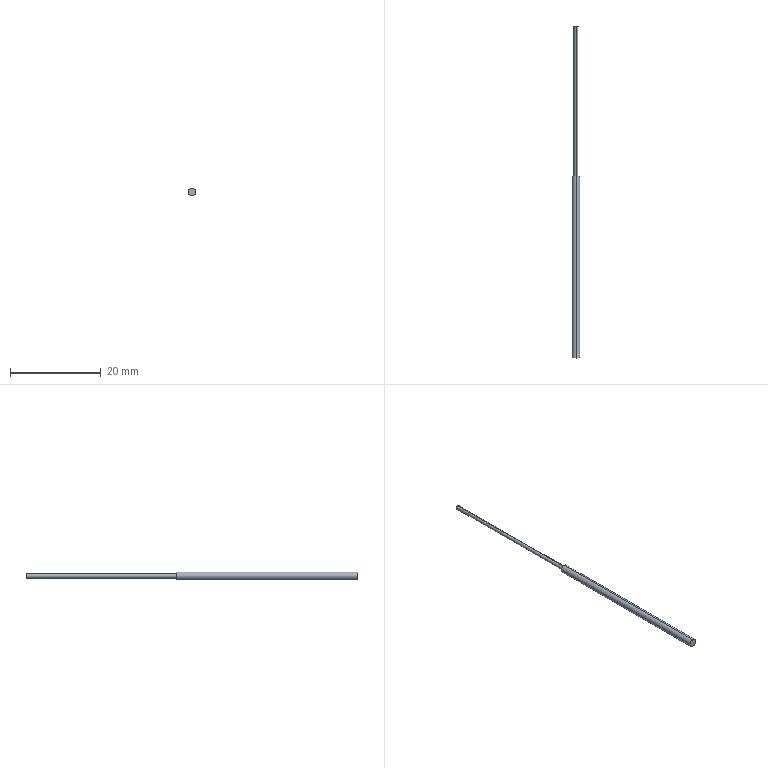Part | SolidWorks | features Extrusion 1, ICE 1 | 1 solid | 7 faces | box 1.75 x 73 x 1.75 mm | volume 117.205 mm3 | cylinder 4 | plane 3 | commonest cylinder face diameters 0.9 x2 1.75 x2
STEP:
#1=CARTESIAN_POINT('',(0.,73.,0.45));
#2=VERTEX_POINT('',#1);
#3=CARTESIAN_POINT('',(0.,73.,-0.45));
#4=VERTEX_POINT('',#3);
#5=CARTESIAN_POINT('',(0.,73.,0.));
#6=DIRECTION('',(0.,1.,0.));
#7=DIRECTION('',(0.,0.,1.));
#8=AXIS2_PLACEMENT_3D('',#5,#6,#7);
#9=CIRCLE('',#8,0.45);
#10=EDGE_CURVE('',#2,#4,#9,.T.);
#11=ORIENTED_EDGE('',*,*,#10,.F.);
#12=CARTESIAN_POINT('',(0.,40.,0.45));
#13=VERTEX_POINT('',#12);
#14=CARTESIAN_POINT('',(0.,73.,0.45));
#15=DIRECTION('',(0.,-1.,0.));
#16=VECTOR('',#15,1000.);
#17=LINE('',#14,#16);
#18=EDGE_CURVE('',#2,#13,#17,.T.);
#19=ORIENTED_EDGE('',*,*,#18,.T.);
#20=CARTESIAN_POINT('',(0.,40.,-0.45));
#21=VERTEX_POINT('',#20);
#22=CARTESIAN_POINT('',(0.,40.,0.));
#23=DIRECTION('',(0.,1.,0.));
#24=DIRECTION('',(0.,0.,1.));
#25=AXIS2_PLACEMENT_3D('',#22,#23,#24);
#26=CIRCLE('',#25,0.45);
#27=EDGE_CURVE('',#13,#21,#26,.T.);
#28=ORIENTED_EDGE('',*,*,#27,.T.);
#29=CARTESIAN_POINT('',(0.,73.,-0.45));
#30=DIRECTION('',(0.,-1.,0.));
#31=VECTOR('',#30,1000.);
#32=LINE('',#29,#31);
#33=EDGE_CURVE('',#4,#21,#32,.T.);
#34=ORIENTED_EDGE('',*,*,#33,.F.);
#35=EDGE_LOOP('',(#11,#19,#28,#34));
#36=FACE_OUTER_BOUND('',#35,.T.);
#37=CARTESIAN_POINT('',(0.,73.,0.));
#38=DIRECTION('',(0.,-1.,0.));
#39=DIRECTION('',(0.,0.,-1.));
#40=AXIS2_PLACEMENT_3D('',#37,#38,#39);
#41=CYLINDRICAL_SURFACE('',#40,0.45);
#42=ADVANCED_FACE('',(#36),#41,.T.);
#43=CARTESIAN_POINT('',(0.,40.,0.875));
#44=VERTEX_POINT('',#43);
#45=CARTESIAN_POINT('',(0.,40.,-0.875));
#46=VERTEX_POINT('',#45);
#47=CARTESIAN_POINT('',(0.,40.,0.));
#48=DIRECTION('',(0.,1.,0.));
#49=DIRECTION('',(0.,0.,1.));
#50=AXIS2_PLACEMENT_3D('',#47,#48,#49);
#51=CIRCLE('',#50,0.875);
#52=EDGE_CURVE('',#44,#46,#51,.T.);
#53=ORIENTED_EDGE('',*,*,#52,.F.);
#54=CARTESIAN_POINT('',(0.,0.,0.875));
#55=VERTEX_POINT('',#54);
#56=CARTESIAN_POINT('',(0.,40.,0.875));
#57=DIRECTION('',(0.,-1.,0.));
#58=VECTOR('',#57,1000.);
#59=LINE('',#56,#58);
#60=EDGE_CURVE('',#44,#55,#59,.T.);
#61=ORIENTED_EDGE('',*,*,#60,.T.);
#62=CARTESIAN_POINT('',(0.,0.,-0.875));
#63=VERTEX_POINT('',#62);
#64=CARTESIAN_POINT('',(0.,0.,0.));
#65=DIRECTION('',(0.,1.,0.));
#66=DIRECTION('',(0.,0.,1.));
#67=AXIS2_PLACEMENT_3D('',#64,#65,#66);
#68=CIRCLE('',#67,0.875);
#69=EDGE_CURVE('',#55,#63,#68,.T.);
#70=ORIENTED_EDGE('',*,*,#69,.T.);
#71=CARTESIAN_POINT('',(0.,40.,-0.875));
#72=DIRECTION('',(0.,-1.,0.));
#73=VECTOR('',#72,1000.);
#74=LINE('',#71,#73);
#75=EDGE_CURVE('',#46,#63,#74,.T.);
#76=ORIENTED_EDGE('',*,*,#75,.F.);
#77=EDGE_LOOP('',(#53,#61,#70,#76));
#78=FACE_OUTER_BOUND('',#77,.T.);
#79=CARTESIAN_POINT('',(0.,40.,0.));
#80=DIRECTION('',(0.,-1.,0.));
#81=DIRECTION('',(0.,0.,-1.));
#82=AXIS2_PLACEMENT_3D('',#79,#80,#81);
#83=CYLINDRICAL_SURFACE('',#82,0.875);
#84=ADVANCED_FACE('',(#78),#83,.T.);
#85=CARTESIAN_POINT('',(0.,40.,0.));
#86=DIRECTION('',(0.,1.,0.));
#87=DIRECTION('',(0.,0.,1.));
#88=AXIS2_PLACEMENT_3D('',#85,#86,#87);
#89=CIRCLE('',#88,0.875);
#90=EDGE_CURVE('',#46,#44,#89,.T.);
#91=ORIENTED_EDGE('',*,*,#90,.T.);
#92=ORIENTED_EDGE('',*,*,#52,.T.);
#93=EDGE_LOOP('',(#91,#92));
#94=FACE_OUTER_BOUND('',#93,.T.);
#95=CARTESIAN_POINT('',(0.,40.,0.));
#96=DIRECTION('',(0.,1.,0.));
#97=DIRECTION('',(0.,0.,1.));
#98=AXIS2_PLACEMENT_3D('',#95,#96,#97);
#99=CIRCLE('',#98,0.45);
#100=EDGE_CURVE('',#21,#13,#99,.T.);
#101=ORIENTED_EDGE('',*,*,#100,.F.);
#102=ORIENTED_EDGE('',*,*,#27,.F.);
#103=EDGE_LOOP('',(#101,#102));
#104=FACE_BOUND('',#103,.T.);
#105=CARTESIAN_POINT('',(0.,40.,0.));
#106=DIRECTION('',(0.,1.,0.));
#107=DIRECTION('',(0.,0.,1.));
#108=AXIS2_PLACEMENT_3D('',#105,#106,#107);
#109=PLANE('',#108);
#110=ADVANCED_FACE('',(#94,#104),#109,.T.);
#111=ORIENTED_EDGE('',*,*,#60,.F.);
#112=ORIENTED_EDGE('',*,*,#90,.F.);
#113=ORIENTED_EDGE('',*,*,#75,.T.);
#114=CARTESIAN_POINT('',(0.,0.,0.));
#115=DIRECTION('',(0.,1.,0.));
#116=DIRECTION('',(0.,0.,1.));
#117=AXIS2_PLACEMENT_3D('',#114,#115,#116);
#118=CIRCLE('',#117,0.875);
#119=EDGE_CURVE('',#63,#55,#118,.T.);
#120=ORIENTED_EDGE('',*,*,#119,.T.);
#121=EDGE_LOOP('',(#111,#112,#113,#120));
#122=FACE_OUTER_BOUND('',#121,.T.);
#123=CARTESIAN_POINT('',(0.,40.,0.));
#124=DIRECTION('',(0.,-1.,0.));
#125=DIRECTION('',(0.,0.,-1.));
#126=AXIS2_PLACEMENT_3D('',#123,#124,#125);
#127=CYLINDRICAL_SURFACE('',#126,0.875);
#128=ADVANCED_FACE('',(#122),#127,.T.);
#129=ORIENTED_EDGE('',*,*,#119,.F.);
#130=ORIENTED_EDGE('',*,*,#69,.F.);
#131=EDGE_LOOP('',(#129,#130));
#132=FACE_OUTER_BOUND('',#131,.T.);
#133=CARTESIAN_POINT('',(0.,0.,0.));
#134=DIRECTION('',(0.,1.,0.));
#135=DIRECTION('',(0.,0.,1.));
#136=AXIS2_PLACEMENT_3D('',#133,#134,#135);
#137=PLANE('',#136);
#138=ADVANCED_FACE('',(#132),#137,.F.);
#139=ORIENTED_EDGE('',*,*,#18,.F.);
#140=CARTESIAN_POINT('',(0.,73.,0.));
#141=DIRECTION('',(0.,1.,0.));
#142=DIRECTION('',(0.,0.,1.));
#143=AXIS2_PLACEMENT_3D('',#140,#141,#142);
#144=CIRCLE('',#143,0.45);
#145=EDGE_CURVE('',#4,#2,#144,.T.);
#146=ORIENTED_EDGE('',*,*,#145,.F.);
#147=ORIENTED_EDGE('',*,*,#33,.T.);
#148=ORIENTED_EDGE('',*,*,#100,.T.);
#149=EDGE_LOOP('',(#139,#146,#147,#148));
#150=FACE_OUTER_BOUND('',#149,.T.);
#151=CARTESIAN_POINT('',(0.,73.,0.));
#152=DIRECTION('',(0.,-1.,0.));
#153=DIRECTION('',(0.,0.,-1.));
#154=AXIS2_PLACEMENT_3D('',#151,#152,#153);
#155=CYLINDRICAL_SURFACE('',#154,0.45);
#156=ADVANCED_FACE('',(#150),#155,.T.);
#157=ORIENTED_EDGE('',*,*,#145,.T.);
#158=ORIENTED_EDGE('',*,*,#10,.T.);
#159=EDGE_LOOP('',(#157,#158));
#160=FACE_OUTER_BOUND('',#159,.T.);
#161=CARTESIAN_POINT('',(0.,73.,0.));
#162=DIRECTION('',(0.,1.,0.));
#163=DIRECTION('',(0.,0.,1.));
#164=AXIS2_PLACEMENT_3D('',#161,#162,#163);
#165=PLANE('',#164);
#166=ADVANCED_FACE('',(#160),#165,.T.);
#167=CLOSED_SHELL('',(#42,#84,#110,#128,#138,#156,#166));
#168=MANIFOLD_SOLID_BREP('',#167);
#169=CARTESIAN_POINT('',(0.,0.,0.));
#170=DIRECTION('',(0.,0.,1.));
#171=DIRECTION('',(1.,0.,0.));
#172=AXIS2_PLACEMENT_3D('',#169,#170,#171);
#173=(LENGTH_UNIT()NAMED_UNIT(*)SI_UNIT(.MILLI.,.METRE.));
#174=UNCERTAINTY_MEASURE_WITH_UNIT(LENGTH_MEASURE(0.00001),#173,'','');
#175=(NAMED_UNIT(*)PLANE_ANGLE_UNIT()SI_UNIT($,.RADIAN.));
#176=(NAMED_UNIT(*)SI_UNIT($,.STERADIAN.)SOLID_ANGLE_UNIT());
#177=(GEOMETRIC_REPRESENTATION_CONTEXT(3)GLOBAL_UNCERTAINTY_ASSIGNED_CONTEXT((#174))GLOBAL_UNIT_ASSIGNED_CONTEXT((#173,#175,#176))REPRESENTATION_CONTEXT('',''));
#178=ADVANCED_BREP_SHAPE_REPRESENTATION('',(#168,#172),#177);